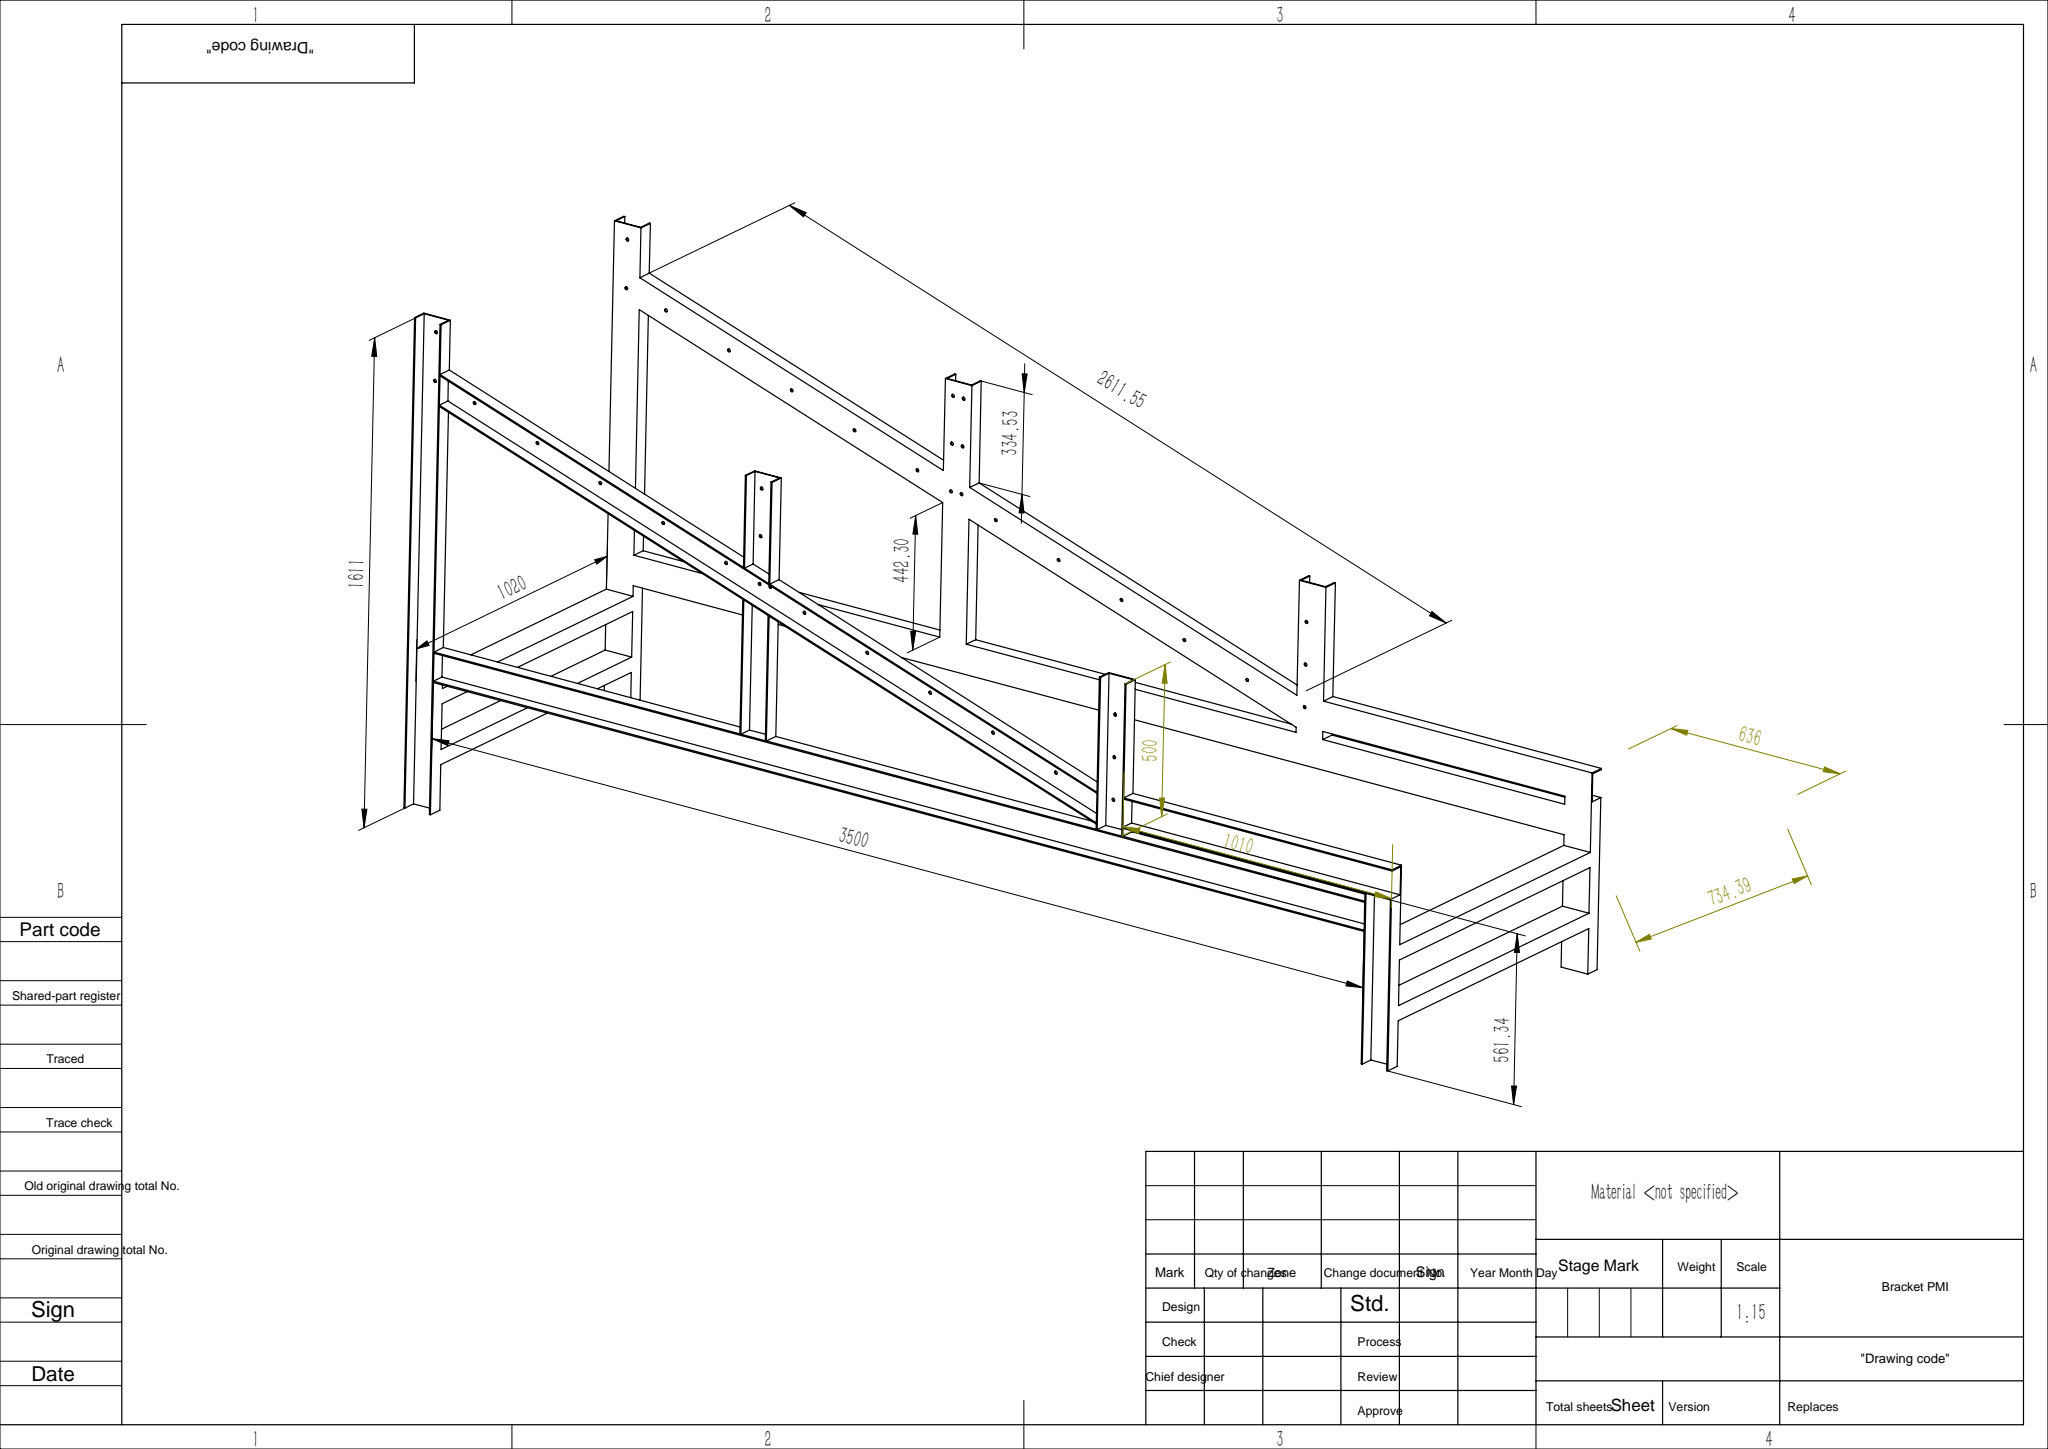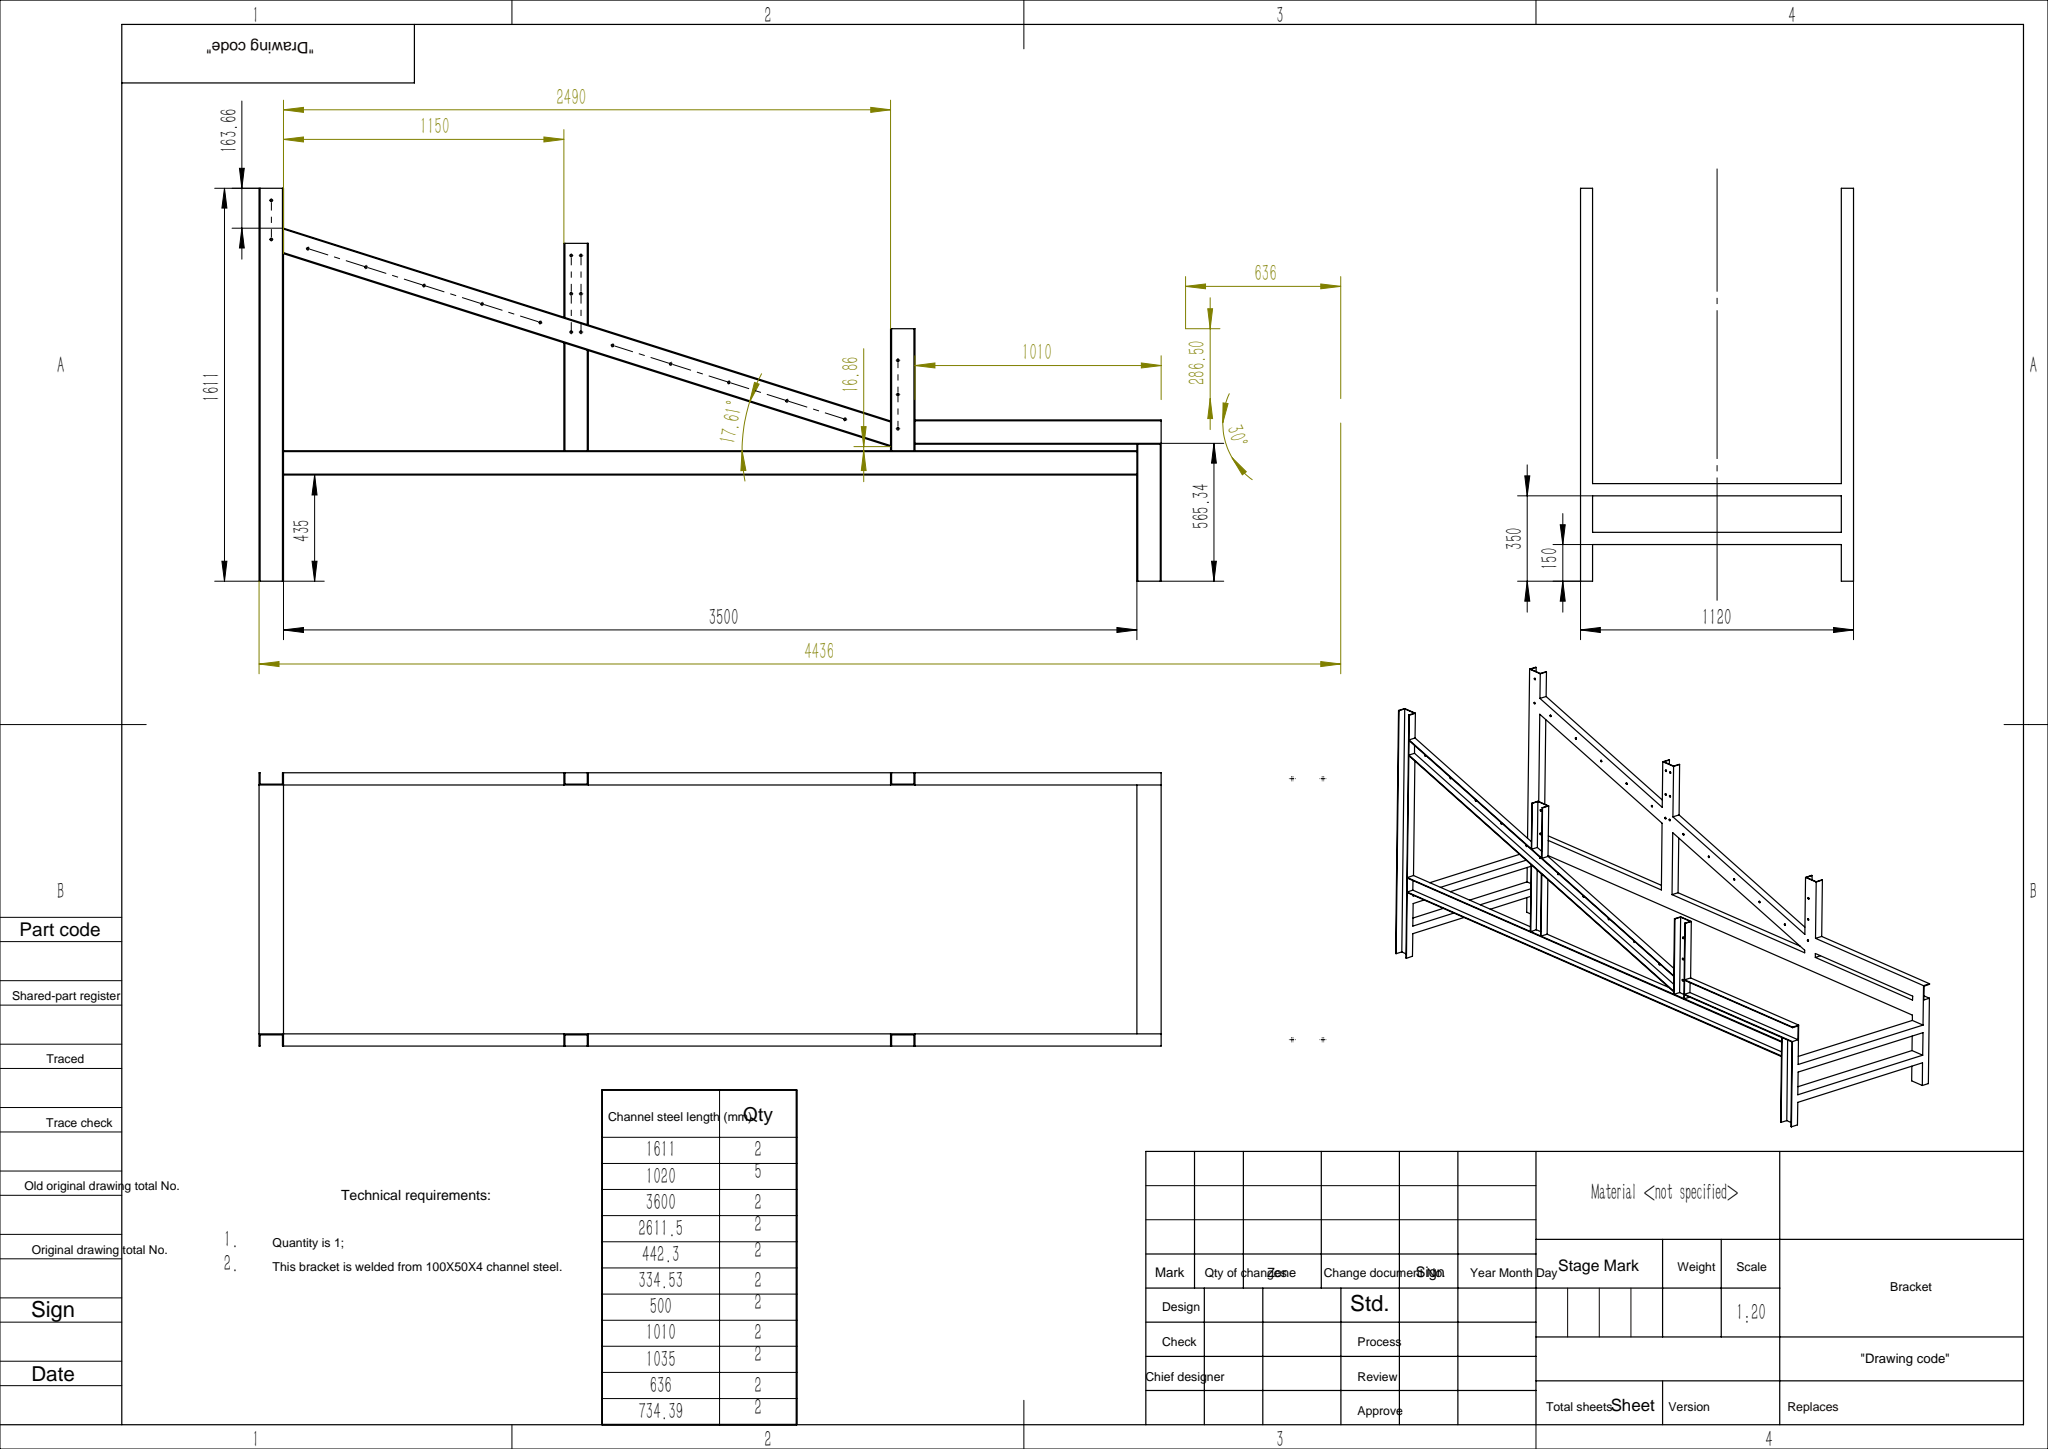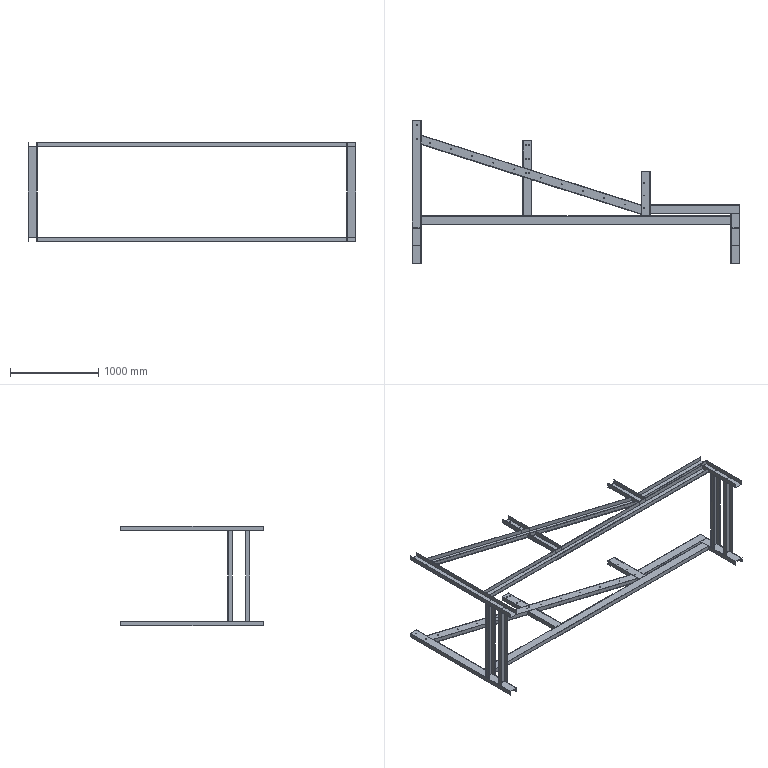Part | SolidWorks | features ICE 8, Cut 6, LPattern 6, Extrusion 1, MirrorPattern 1 | 1 solid | 246 faces | box 3700 x 1611 x 1120 mm | volume 19309543 mm3 | plane 162 | cylinder 84 | commonest cylinder face diameters 10 x84